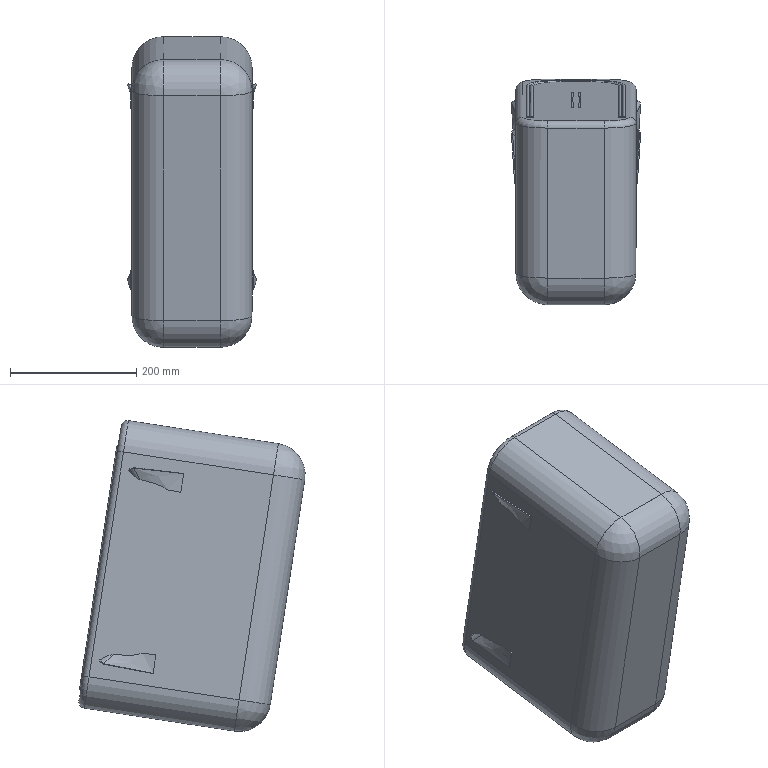Part | SolidWorks | features BaseBody 1 | 1 solid | 219 faces | box 204.557 x 357.856 x 491.744 mm | volume 1059121 mm3 | spline 148 | cylinder 37 | torus 14 | plane 12 | sphere 8 | commonest cylinder face diameters 4 x13 96 x8 100 x8 16 x4 20 x4